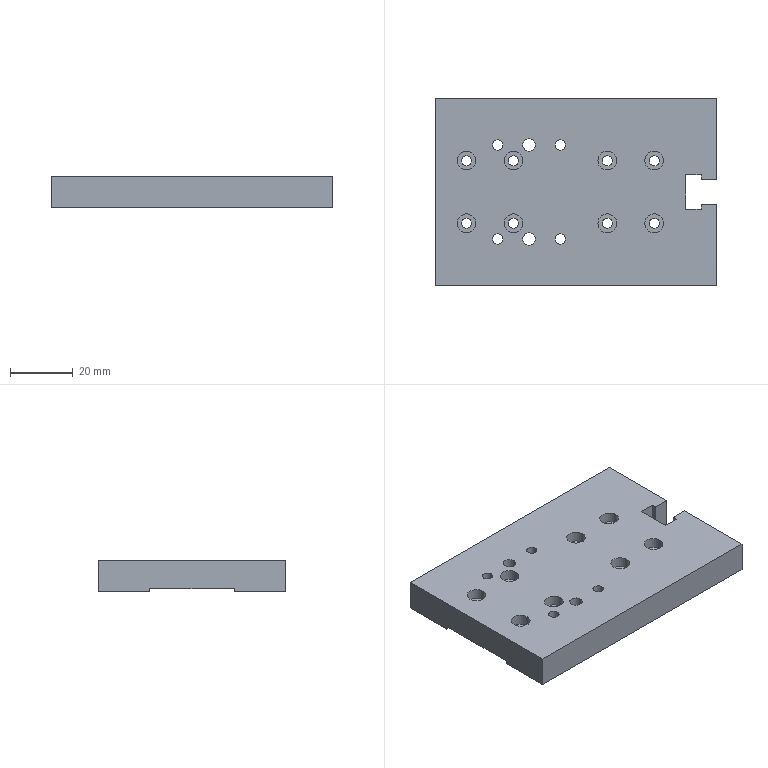Part | STEP file | 2078 Slider mounting plate | 1 solid | 76 faces | box 90 x 60 x 10 mm | volume 48995 mm3 | cylinder 44 | plane 32 | commonest cylinder face diameters 3.2 x16 6 x16 3.3 x8 4 x4